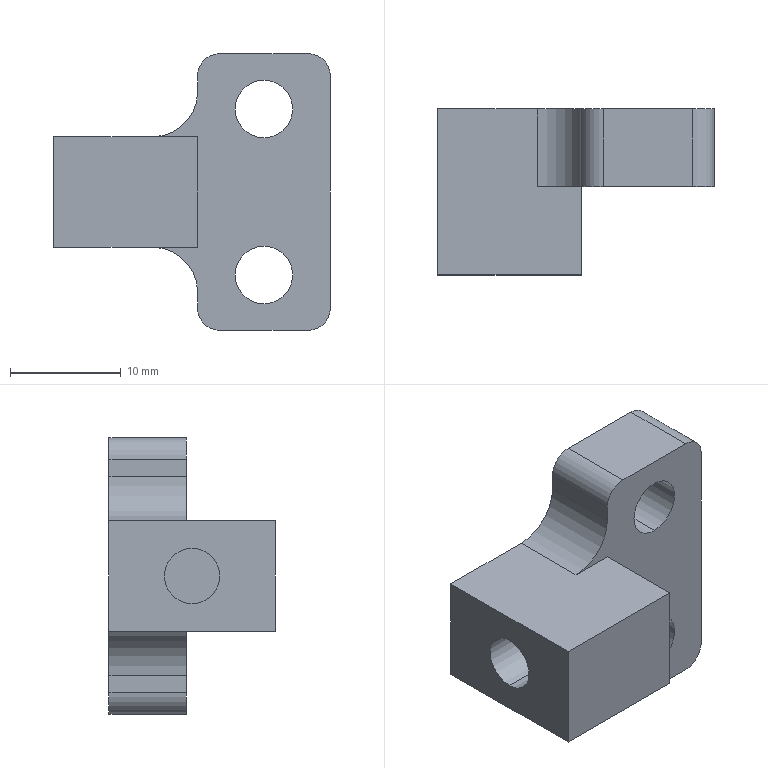CAM job | Mastercam | 3-axis milling, drilling | stock box 35 x 15 x 35 mm
Tools:
tool_number,name,type,diameter_mm,corner_radius_mm,flutes,flute_length_mm,overall_length_mm,shoulder_length_mm,holder_diameter_mm,length_offset,diameter_offset,default_rpm,default_feed_mm_min,default_plunge_mm_min,coolant
6,6 Flat End Mill,end mill,6,0,4,25,75,25,50,6,6,3500,500,600,COOL_OFF
6,6 Flat End Mill,end mill,6,0,4,6,12,7.2,50,6,6,7003,840.36,1000,COOL_OFF
7,4 Chamfer Mill,chamfer mill,4,0,4,25,75,30,50,7,7,3000,300,600,COOL_OFF
8,8 Flat End Mill,end mill,8,0,4,25,75,25,50,8,8,7000,3000,600,COOL_OFF
24,63 Flat End Mill,end mill,63,0,4,25,75,25,50,24,24,4000,1000,600,COOL_OFF
Operations:
seq,operation,operation_type,tool_number,tool_name,tool_diameter_mm,spindle_rpm,feed_mm_min,plunge_mm_min,retract_mm_min,cycle_time_s,wcs,posted,nc_file
1,Facing - [WCS: Plane] - [Tplane: Plane],Facing,24,63 Flat End Mill,63,4000,1000,600,1200,11.086,Plane,yes,.nc
2,3D High Speed (Dynamic OptiRough) - [WCS: Plane] - [Tplane: Plane],HighSpeed3D,8,8 Flat End Mill,8,7000,3000,600,1200,106.613,Plane,yes,.nc
3,Contour (2D) - [WCS: Plane] - [Tplane: Plane],Contour,6,6 Flat End Mill,6,7000,1000,600,1200,6.745,Plane,yes,.nc
4,2D High Speed (2D Area Mill) - [WCS: Plane] - [Tplane: Plane],HighSpeed2D,6,6 Flat End Mill,6,7000,500,600,1200,18.484,Plane,yes,.nc
5,Contour (2D) - [WCS: Plane] - [Tplane: Plane],Contour,6,6 Flat End Mill,6,7000,1000,600,1200,17.977,Plane,yes,.nc
6,Drill/Counterbore - [WCS: Plane] - [Tplane: Plane],Drill,7,4 Chamfer Mill,4,3000,300,600,1200,1.637,Plane,yes,.nc
7,Model Chamfer - [WCS: Plane] - [Tplane: Plane],ModelChamfer,7,4 Chamfer Mill,4,7000,1000,1000,2000,7.862,Plane,yes,.nc
8,Facing - [WCS: Plane-1] - [Tplane: Plane-1],Facing,24,63 Flat End Mill,63,4000,3000,600,1200,45.855,Plane-1,yes,.nc
9,Contour (2D chamfer) - [WCS: Plane-1] - [Tplane: Plane-1],Contour,7,4 Chamfer Mill,4,7000,1000,600,1200,6.615,Plane-1,yes,.nc